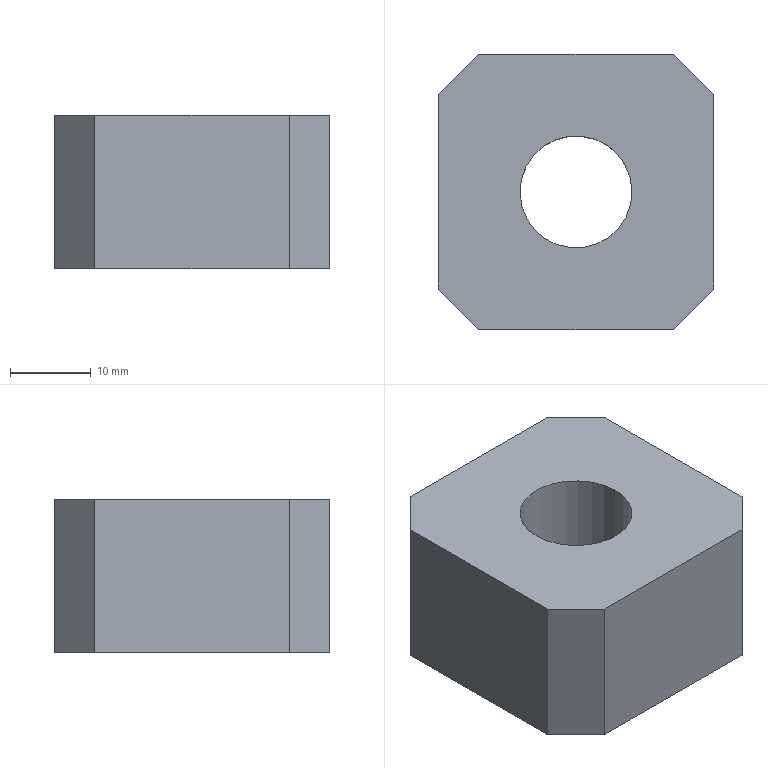Part | STEP file | SN10_002_008-07_PLACA | 1 solid | 11 faces | box 34 x 34 x 19 mm | volume 18158 mm3 | plane 10 | cylinder 1 | commonest cylinder face diameters 13.835 x1
STEP:
#1=CARTESIAN_POINT('',(0.,0.,0.));
#2=DIRECTION('',(0.,0.,1.));
#3=DIRECTION('',(1.,0.,0.));
#4=AXIS2_PLACEMENT_3D('',#1,#2,#3);
#5=CARTESIAN_POINT('',(6.071,3.316,-19.));
#6=VERTEX_POINT('',#5);
#7=CARTESIAN_POINT('',(0.,0.,-19.));
#8=DIRECTION('',(0.,0.,1.));
#9=DIRECTION('',(1.,0.,0.));
#10=AXIS2_PLACEMENT_3D('',#7,#8,#9);
#11=CIRCLE('',#10,6.918);
#12=CARTESIAN_POINT('',(0.,0.,-18.9));
#13=DIRECTION('',(0.,0.,1.));
#14=DIRECTION('',(0.8776,0.4794,0.));
#15=AXIS2_PLACEMENT_3D('',#12,#13,#14);
#16=CYLINDRICAL_SURFACE('',#15,6.918);
#17=CARTESIAN_POINT('',(-0.5,-0.1));
#18=DIRECTION('',(1.,0.));
#19=VECTOR('',#18,1.);
#20=LINE('',#17,#19);
#21=(GEOMETRIC_REPRESENTATION_CONTEXT(2)PARAMETRIC_REPRESENTATION_CONTEXT()REPRESENTATION_CONTEXT('',''));
#22=DEFINITIONAL_REPRESENTATION('',(#20),#21);
#23=PCURVE('',#16,#22);
#24=CARTESIAN_POINT('',(0.,0.,-19.));
#25=DIRECTION('',(0.,0.,1.));
#26=DIRECTION('',(1.,0.,0.));
#27=AXIS2_PLACEMENT_3D('',#24,#25,#26);
#28=PLANE('',#27);
#29=CARTESIAN_POINT('',(0.,0.));
#30=DIRECTION('',(1.,0.));
#31=AXIS2_PLACEMENT_2D('',#29,#30);
#32=CIRCLE('',#31,6.918);
#33=(GEOMETRIC_REPRESENTATION_CONTEXT(2)PARAMETRIC_REPRESENTATION_CONTEXT()REPRESENTATION_CONTEXT('',''));
#34=DEFINITIONAL_REPRESENTATION('',(#32),#33);
#35=PCURVE('',#28,#34);
#36=SURFACE_CURVE('',#11,(#23,#35),.PCURVE_S1.);
#37=EDGE_CURVE('',#6,#6,#36,.T.);
#38=ORIENTED_EDGE('',*,*,#37,.T.);
#39=CARTESIAN_POINT('',(6.071,3.316,0.));
#40=VERTEX_POINT('',#39);
#41=CARTESIAN_POINT('',(6.071,3.316,-19.));
#42=CARTESIAN_POINT('',(6.071,3.316,0.));
#43=B_SPLINE_CURVE_WITH_KNOTS('',1,(#41,#42),.UNSPECIFIED.,.F.,.F.,(2,2),(-0.1,18.9),.PIECEWISE_BEZIER_KNOTS.);
#44=CARTESIAN_POINT('',(6.283,0.));
#45=DIRECTION('',(0.,1.));
#46=VECTOR('',#45,1.);
#47=LINE('',#44,#46);
#48=(GEOMETRIC_REPRESENTATION_CONTEXT(2)PARAMETRIC_REPRESENTATION_CONTEXT()REPRESENTATION_CONTEXT('',''));
#49=DEFINITIONAL_REPRESENTATION('',(#47),#48);
#50=PCURVE('',#16,#49);
#51=CARTESIAN_POINT('',(0.,0.));
#52=DIRECTION('',(0.,1.));
#53=VECTOR('',#52,1.);
#54=LINE('',#51,#53);
#55=(GEOMETRIC_REPRESENTATION_CONTEXT(2)PARAMETRIC_REPRESENTATION_CONTEXT()REPRESENTATION_CONTEXT('',''));
#56=DEFINITIONAL_REPRESENTATION('',(#54),#55);
#57=PCURVE('',#16,#56);
#58=SEAM_CURVE('',#43,(#50,#57),.PCURVE_S1.);
#59=EDGE_CURVE('',#6,#40,#58,.T.);
#60=ORIENTED_EDGE('',*,*,#59,.T.);
#61=CARTESIAN_POINT('',(0.,0.,0.));
#62=DIRECTION('',(0.,0.,1.));
#63=DIRECTION('',(1.,0.,0.));
#64=AXIS2_PLACEMENT_3D('',#61,#62,#63);
#65=CIRCLE('',#64,6.918);
#66=CARTESIAN_POINT('',(-0.5,18.9));
#67=DIRECTION('',(1.,0.));
#68=VECTOR('',#67,1.);
#69=LINE('',#66,#68);
#70=(GEOMETRIC_REPRESENTATION_CONTEXT(2)PARAMETRIC_REPRESENTATION_CONTEXT()REPRESENTATION_CONTEXT('',''));
#71=DEFINITIONAL_REPRESENTATION('',(#69),#70);
#72=PCURVE('',#16,#71);
#73=CARTESIAN_POINT('',(0.,0.,0.));
#74=DIRECTION('',(0.,0.,1.));
#75=DIRECTION('',(1.,0.,0.));
#76=AXIS2_PLACEMENT_3D('',#73,#74,#75);
#77=PLANE('',#76);
#78=CARTESIAN_POINT('',(0.,0.));
#79=DIRECTION('',(1.,0.));
#80=AXIS2_PLACEMENT_2D('',#78,#79);
#81=CIRCLE('',#80,6.918);
#82=(GEOMETRIC_REPRESENTATION_CONTEXT(2)PARAMETRIC_REPRESENTATION_CONTEXT()REPRESENTATION_CONTEXT('',''));
#83=DEFINITIONAL_REPRESENTATION('',(#81),#82);
#84=PCURVE('',#77,#83);
#85=SURFACE_CURVE('',#65,(#72,#84),.PCURVE_S1.);
#86=EDGE_CURVE('',#40,#40,#85,.T.);
#87=ORIENTED_EDGE('',*,*,#86,.F.);
#88=ORIENTED_EDGE('',*,*,#59,.F.);
#89=EDGE_LOOP('',(#38,#60,#87,#88));
#90=FACE_BOUND('',#89,.F.);
#91=ADVANCED_FACE('',(#90),#16,.F.);
#92=CARTESIAN_POINT('',(-17.,-12.,0.));
#93=VERTEX_POINT('',#92);
#94=CARTESIAN_POINT('',(-17.,12.,0.));
#95=VERTEX_POINT('',#94);
#96=CARTESIAN_POINT('',(-17.,-12.,0.));
#97=DIRECTION('',(0.,1.,0.));
#98=VECTOR('',#97,1.);
#99=LINE('',#96,#98);
#100=CARTESIAN_POINT('',(-17.,-12.));
#101=DIRECTION('',(0.,1.));
#102=VECTOR('',#101,1.);
#103=LINE('',#100,#102);
#104=(GEOMETRIC_REPRESENTATION_CONTEXT(2)PARAMETRIC_REPRESENTATION_CONTEXT()REPRESENTATION_CONTEXT('',''));
#105=DEFINITIONAL_REPRESENTATION('',(#103),#104);
#106=PCURVE('',#77,#105);
#107=CARTESIAN_POINT('',(-17.,-17.,0.));
#108=DIRECTION('',(-1.,0.,0.));
#109=DIRECTION('',(0.,0.,1.));
#110=AXIS2_PLACEMENT_3D('',#107,#108,#109);
#111=PLANE('',#110);
#112=CARTESIAN_POINT('',(0.,5.));
#113=DIRECTION('',(0.,1.));
#114=VECTOR('',#113,1.);
#115=LINE('',#112,#114);
#116=(GEOMETRIC_REPRESENTATION_CONTEXT(2)PARAMETRIC_REPRESENTATION_CONTEXT()REPRESENTATION_CONTEXT('',''));
#117=DEFINITIONAL_REPRESENTATION('',(#115),#116);
#118=PCURVE('',#111,#117);
#119=SURFACE_CURVE('',#99,(#106,#118),.PCURVE_S1.);
#120=EDGE_CURVE('',#93,#95,#119,.T.);
#121=ORIENTED_EDGE('',*,*,#120,.F.);
#122=CARTESIAN_POINT('',(-12.,-17.,0.));
#123=VERTEX_POINT('',#122);
#124=CARTESIAN_POINT('',(-17.,-12.,0.));
#125=DIRECTION('',(0.7071,-0.7071,0.));
#126=VECTOR('',#125,1.);
#127=LINE('',#124,#126);
#128=CARTESIAN_POINT('',(-17.,-12.));
#129=DIRECTION('',(0.7071,-0.7071));
#130=VECTOR('',#129,1.);
#131=LINE('',#128,#130);
#132=(GEOMETRIC_REPRESENTATION_CONTEXT(2)PARAMETRIC_REPRESENTATION_CONTEXT()REPRESENTATION_CONTEXT('',''));
#133=DEFINITIONAL_REPRESENTATION('',(#131),#132);
#134=PCURVE('',#77,#133);
#135=CARTESIAN_POINT('',(-17.,-12.,-22.8));
#136=DIRECTION('',(0.7071,0.7071,0.));
#137=DIRECTION('',(0.,0.,-1.));
#138=AXIS2_PLACEMENT_3D('',#135,#136,#137);
#139=PLANE('',#138);
#140=CARTESIAN_POINT('',(-22.8,0.));
#141=DIRECTION('',(0.,-1.));
#142=VECTOR('',#141,1.);
#143=LINE('',#140,#142);
#144=(GEOMETRIC_REPRESENTATION_CONTEXT(2)PARAMETRIC_REPRESENTATION_CONTEXT()REPRESENTATION_CONTEXT('',''));
#145=DEFINITIONAL_REPRESENTATION('',(#143),#144);
#146=PCURVE('',#139,#145);
#147=SURFACE_CURVE('',#127,(#134,#146),.PCURVE_S1.);
#148=EDGE_CURVE('',#93,#123,#147,.T.);
#149=ORIENTED_EDGE('',*,*,#148,.T.);
#150=CARTESIAN_POINT('',(12.,-17.,0.));
#151=VERTEX_POINT('',#150);
#152=CARTESIAN_POINT('',(12.,-17.,0.));
#153=DIRECTION('',(-1.,0.,0.));
#154=VECTOR('',#153,1.);
#155=LINE('',#152,#154);
#156=CARTESIAN_POINT('',(12.,-17.));
#157=DIRECTION('',(-1.,0.));
#158=VECTOR('',#157,1.);
#159=LINE('',#156,#158);
#160=(GEOMETRIC_REPRESENTATION_CONTEXT(2)PARAMETRIC_REPRESENTATION_CONTEXT()REPRESENTATION_CONTEXT('',''));
#161=DEFINITIONAL_REPRESENTATION('',(#159),#160);
#162=PCURVE('',#77,#161);
#163=CARTESIAN_POINT('',(17.,-17.,0.));
#164=DIRECTION('',(0.,-1.,0.));
#165=DIRECTION('',(0.,0.,-1.));
#166=AXIS2_PLACEMENT_3D('',#163,#164,#165);
#167=PLANE('',#166);
#168=CARTESIAN_POINT('',(0.,-5.));
#169=DIRECTION('',(0.,-1.));
#170=VECTOR('',#169,1.);
#171=LINE('',#168,#170);
#172=(GEOMETRIC_REPRESENTATION_CONTEXT(2)PARAMETRIC_REPRESENTATION_CONTEXT()REPRESENTATION_CONTEXT('',''));
#173=DEFINITIONAL_REPRESENTATION('',(#171),#172);
#174=PCURVE('',#167,#173);
#175=SURFACE_CURVE('',#155,(#162,#174),.PCURVE_S1.);
#176=EDGE_CURVE('',#151,#123,#175,.T.);
#177=ORIENTED_EDGE('',*,*,#176,.F.);
#178=CARTESIAN_POINT('',(17.,-12.,0.));
#179=VERTEX_POINT('',#178);
#180=CARTESIAN_POINT('',(17.,-12.,0.));
#181=DIRECTION('',(-0.7071,-0.7071,0.));
#182=VECTOR('',#181,1.);
#183=LINE('',#180,#182);
#184=CARTESIAN_POINT('',(17.,-12.));
#185=DIRECTION('',(-0.7071,-0.7071));
#186=VECTOR('',#185,1.);
#187=LINE('',#184,#186);
#188=(GEOMETRIC_REPRESENTATION_CONTEXT(2)PARAMETRIC_REPRESENTATION_CONTEXT()REPRESENTATION_CONTEXT('',''));
#189=DEFINITIONAL_REPRESENTATION('',(#187),#188);
#190=PCURVE('',#77,#189);
#191=CARTESIAN_POINT('',(17.,-12.,3.8));
#192=DIRECTION('',(-0.7071,0.7071,0.));
#193=DIRECTION('',(0.,0.,1.));
#194=AXIS2_PLACEMENT_3D('',#191,#192,#193);
#195=PLANE('',#194);
#196=CARTESIAN_POINT('',(-3.8,0.));
#197=DIRECTION('',(0.,-1.));
#198=VECTOR('',#197,1.);
#199=LINE('',#196,#198);
#200=(GEOMETRIC_REPRESENTATION_CONTEXT(2)PARAMETRIC_REPRESENTATION_CONTEXT()REPRESENTATION_CONTEXT('',''));
#201=DEFINITIONAL_REPRESENTATION('',(#199),#200);
#202=PCURVE('',#195,#201);
#203=SURFACE_CURVE('',#183,(#190,#202),.PCURVE_S1.);
#204=EDGE_CURVE('',#179,#151,#203,.T.);
#205=ORIENTED_EDGE('',*,*,#204,.F.);
#206=CARTESIAN_POINT('',(17.,12.,0.));
#207=VERTEX_POINT('',#206);
#208=CARTESIAN_POINT('',(17.,12.,0.));
#209=DIRECTION('',(0.,-1.,0.));
#210=VECTOR('',#209,1.);
#211=LINE('',#208,#210);
#212=CARTESIAN_POINT('',(17.,12.));
#213=DIRECTION('',(0.,-1.));
#214=VECTOR('',#213,1.);
#215=LINE('',#212,#214);
#216=(GEOMETRIC_REPRESENTATION_CONTEXT(2)PARAMETRIC_REPRESENTATION_CONTEXT()REPRESENTATION_CONTEXT('',''));
#217=DEFINITIONAL_REPRESENTATION('',(#215),#216);
#218=PCURVE('',#77,#217);
#219=CARTESIAN_POINT('',(17.,17.,0.));
#220=DIRECTION('',(1.,0.,0.));
#221=DIRECTION('',(0.,0.,-1.));
#222=AXIS2_PLACEMENT_3D('',#219,#220,#221);
#223=PLANE('',#222);
#224=CARTESIAN_POINT('',(0.,-5.));
#225=DIRECTION('',(0.,-1.));
#226=VECTOR('',#225,1.);
#227=LINE('',#224,#226);
#228=(GEOMETRIC_REPRESENTATION_CONTEXT(2)PARAMETRIC_REPRESENTATION_CONTEXT()REPRESENTATION_CONTEXT('',''));
#229=DEFINITIONAL_REPRESENTATION('',(#227),#228);
#230=PCURVE('',#223,#229);
#231=SURFACE_CURVE('',#211,(#218,#230),.PCURVE_S1.);
#232=EDGE_CURVE('',#207,#179,#231,.T.);
#233=ORIENTED_EDGE('',*,*,#232,.F.);
#234=CARTESIAN_POINT('',(12.,17.,0.));
#235=VERTEX_POINT('',#234);
#236=CARTESIAN_POINT('',(12.,17.,0.));
#237=DIRECTION('',(0.7071,-0.7071,0.));
#238=VECTOR('',#237,1.);
#239=LINE('',#236,#238);
#240=CARTESIAN_POINT('',(12.,17.));
#241=DIRECTION('',(0.7071,-0.7071));
#242=VECTOR('',#241,1.);
#243=LINE('',#240,#242);
#244=(GEOMETRIC_REPRESENTATION_CONTEXT(2)PARAMETRIC_REPRESENTATION_CONTEXT()REPRESENTATION_CONTEXT('',''));
#245=DEFINITIONAL_REPRESENTATION('',(#243),#244);
#246=PCURVE('',#77,#245);
#247=CARTESIAN_POINT('',(17.,12.,-22.8));
#248=DIRECTION('',(-0.7071,-0.7071,0.));
#249=DIRECTION('',(0.,0.,1.));
#250=AXIS2_PLACEMENT_3D('',#247,#248,#249);
#251=PLANE('',#250);
#252=CARTESIAN_POINT('',(22.8,7.071));
#253=DIRECTION('',(0.,-1.));
#254=VECTOR('',#253,1.);
#255=LINE('',#252,#254);
#256=(GEOMETRIC_REPRESENTATION_CONTEXT(2)PARAMETRIC_REPRESENTATION_CONTEXT()REPRESENTATION_CONTEXT('',''));
#257=DEFINITIONAL_REPRESENTATION('',(#255),#256);
#258=PCURVE('',#251,#257);
#259=SURFACE_CURVE('',#239,(#246,#258),.PCURVE_S1.);
#260=EDGE_CURVE('',#235,#207,#259,.T.);
#261=ORIENTED_EDGE('',*,*,#260,.F.);
#262=CARTESIAN_POINT('',(-12.,17.,0.));
#263=VERTEX_POINT('',#262);
#264=CARTESIAN_POINT('',(-12.,17.,0.));
#265=DIRECTION('',(1.,0.,0.));
#266=VECTOR('',#265,1.);
#267=LINE('',#264,#266);
#268=CARTESIAN_POINT('',(-12.,17.));
#269=DIRECTION('',(1.,0.));
#270=VECTOR('',#269,1.);
#271=LINE('',#268,#270);
#272=(GEOMETRIC_REPRESENTATION_CONTEXT(2)PARAMETRIC_REPRESENTATION_CONTEXT()REPRESENTATION_CONTEXT('',''));
#273=DEFINITIONAL_REPRESENTATION('',(#271),#272);
#274=PCURVE('',#77,#273);
#275=CARTESIAN_POINT('',(-17.,17.,0.));
#276=DIRECTION('',(0.,1.,0.));
#277=DIRECTION('',(0.,0.,1.));
#278=AXIS2_PLACEMENT_3D('',#275,#276,#277);
#279=PLANE('',#278);
#280=CARTESIAN_POINT('',(0.,5.));
#281=DIRECTION('',(0.,1.));
#282=VECTOR('',#281,1.);
#283=LINE('',#280,#282);
#284=(GEOMETRIC_REPRESENTATION_CONTEXT(2)PARAMETRIC_REPRESENTATION_CONTEXT()REPRESENTATION_CONTEXT('',''));
#285=DEFINITIONAL_REPRESENTATION('',(#283),#284);
#286=PCURVE('',#279,#285);
#287=SURFACE_CURVE('',#267,(#274,#286),.PCURVE_S1.);
#288=EDGE_CURVE('',#263,#235,#287,.T.);
#289=ORIENTED_EDGE('',*,*,#288,.F.);
#290=CARTESIAN_POINT('',(-17.,12.,0.));
#291=DIRECTION('',(0.7071,0.7071,0.));
#292=VECTOR('',#291,1.);
#293=LINE('',#290,#292);
#294=CARTESIAN_POINT('',(-17.,12.));
#295=DIRECTION('',(0.7071,0.7071));
#296=VECTOR('',#295,1.);
#297=LINE('',#294,#296);
#298=(GEOMETRIC_REPRESENTATION_CONTEXT(2)PARAMETRIC_REPRESENTATION_CONTEXT()REPRESENTATION_CONTEXT('',''));
#299=DEFINITIONAL_REPRESENTATION('',(#297),#298);
#300=PCURVE('',#77,#299);
#301=CARTESIAN_POINT('',(-17.,12.,3.8));
#302=DIRECTION('',(0.7071,-0.7071,0.));
#303=DIRECTION('',(0.,0.,-1.));
#304=AXIS2_PLACEMENT_3D('',#301,#302,#303);
#305=PLANE('',#304);
#306=CARTESIAN_POINT('',(3.8,0.));
#307=DIRECTION('',(0.,1.));
#308=VECTOR('',#307,1.);
#309=LINE('',#306,#308);
#310=(GEOMETRIC_REPRESENTATION_CONTEXT(2)PARAMETRIC_REPRESENTATION_CONTEXT()REPRESENTATION_CONTEXT('',''));
#311=DEFINITIONAL_REPRESENTATION('',(#309),#310);
#312=PCURVE('',#305,#311);
#313=SURFACE_CURVE('',#293,(#300,#312),.PCURVE_S1.);
#314=EDGE_CURVE('',#95,#263,#313,.T.);
#315=ORIENTED_EDGE('',*,*,#314,.F.);
#316=EDGE_LOOP('',(#121,#149,#177,#205,#233,#261,#289,#315));
#317=FACE_BOUND('',#316,.T.);
#318=ORIENTED_EDGE('',*,*,#86,.F.);
#319=EDGE_LOOP('',(#318));
#320=FACE_BOUND('',#319,.T.);
#321=ADVANCED_FACE('',(#317,#320),#77,.T.);
#322=CARTESIAN_POINT('',(-17.,-12.,-19.));
#323=VERTEX_POINT('',#322);
#324=CARTESIAN_POINT('',(-17.,12.,-19.));
#325=VERTEX_POINT('',#324);
#326=CARTESIAN_POINT('',(-17.,-12.,-19.));
#327=DIRECTION('',(0.,1.,0.));
#328=VECTOR('',#327,1.);
#329=LINE('',#326,#328);
#330=CARTESIAN_POINT('',(-19.,5.));
#331=DIRECTION('',(0.,1.));
#332=VECTOR('',#331,1.);
#333=LINE('',#330,#332);
#334=(GEOMETRIC_REPRESENTATION_CONTEXT(2)PARAMETRIC_REPRESENTATION_CONTEXT()REPRESENTATION_CONTEXT('',''));
#335=DEFINITIONAL_REPRESENTATION('',(#333),#334);
#336=PCURVE('',#111,#335);
#337=CARTESIAN_POINT('',(-17.,-12.));
#338=DIRECTION('',(0.,1.));
#339=VECTOR('',#338,1.);
#340=LINE('',#337,#339);
#341=(GEOMETRIC_REPRESENTATION_CONTEXT(2)PARAMETRIC_REPRESENTATION_CONTEXT()REPRESENTATION_CONTEXT('',''));
#342=DEFINITIONAL_REPRESENTATION('',(#340),#341);
#343=PCURVE('',#28,#342);
#344=SURFACE_CURVE('',#329,(#336,#343),.PCURVE_S1.);
#345=EDGE_CURVE('',#323,#325,#344,.T.);
#346=ORIENTED_EDGE('',*,*,#345,.F.);
#347=CARTESIAN_POINT('',(-17.,-12.,-19.));
#348=DIRECTION('',(0.,0.,1.));
#349=VECTOR('',#348,1.);
#350=LINE('',#347,#349);
#351=CARTESIAN_POINT('',(-19.,5.));
#352=DIRECTION('',(1.,0.));
#353=VECTOR('',#352,1.);
#354=LINE('',#351,#353);
#355=(GEOMETRIC_REPRESENTATION_CONTEXT(2)PARAMETRIC_REPRESENTATION_CONTEXT()REPRESENTATION_CONTEXT('',''));
#356=DEFINITIONAL_REPRESENTATION('',(#354),#355);
#357=PCURVE('',#111,#356);
#358=CARTESIAN_POINT('',(-3.8,0.));
#359=DIRECTION('',(-1.,0.));
#360=VECTOR('',#359,1.);
#361=LINE('',#358,#360);
#362=(GEOMETRIC_REPRESENTATION_CONTEXT(2)PARAMETRIC_REPRESENTATION_CONTEXT()REPRESENTATION_CONTEXT('',''));
#363=DEFINITIONAL_REPRESENTATION('',(#361),#362);
#364=PCURVE('',#139,#363);
#365=SURFACE_CURVE('',#350,(#357,#364),.PCURVE_S1.);
#366=EDGE_CURVE('',#323,#93,#365,.T.);
#367=ORIENTED_EDGE('',*,*,#366,.T.);
#368=ORIENTED_EDGE('',*,*,#120,.T.);
#369=CARTESIAN_POINT('',(-17.,12.,0.));
#370=DIRECTION('',(0.,0.,-1.));
#371=VECTOR('',#370,1.);
#372=LINE('',#369,#371);
#373=CARTESIAN_POINT('',(0.,29.));
#374=DIRECTION('',(-1.,0.));
#375=VECTOR('',#374,1.);
#376=LINE('',#373,#375);
#377=(GEOMETRIC_REPRESENTATION_CONTEXT(2)PARAMETRIC_REPRESENTATION_CONTEXT()REPRESENTATION_CONTEXT('',''));
#378=DEFINITIONAL_REPRESENTATION('',(#376),#377);
#379=PCURVE('',#111,#378);
#380=CARTESIAN_POINT('',(3.8,0.));
#381=DIRECTION('',(1.,0.));
#382=VECTOR('',#381,1.);
#383=LINE('',#380,#382);
#384=(GEOMETRIC_REPRESENTATION_CONTEXT(2)PARAMETRIC_REPRESENTATION_CONTEXT()REPRESENTATION_CONTEXT('',''));
#385=DEFINITIONAL_REPRESENTATION('',(#383),#384);
#386=PCURVE('',#305,#385);
#387=SURFACE_CURVE('',#372,(#379,#386),.PCURVE_S1.);
#388=EDGE_CURVE('',#95,#325,#387,.T.);
#389=ORIENTED_EDGE('',*,*,#388,.T.);
#390=EDGE_LOOP('',(#346,#367,#368,#389));
#391=FACE_BOUND('',#390,.T.);
#392=ADVANCED_FACE('',(#391),#111,.T.);
#393=CARTESIAN_POINT('',(12.,-17.,-19.));
#394=VERTEX_POINT('',#393);
#395=CARTESIAN_POINT('',(-12.,-17.,-19.));
#396=VERTEX_POINT('',#395);
#397=CARTESIAN_POINT('',(12.,-17.,-19.));
#398=DIRECTION('',(-1.,0.,0.));
#399=VECTOR('',#398,1.);
#400=LINE('',#397,#399);
#401=CARTESIAN_POINT('',(19.,-5.));
#402=DIRECTION('',(0.,-1.));
#403=VECTOR('',#402,1.);
#404=LINE('',#401,#403);
#405=(GEOMETRIC_REPRESENTATION_CONTEXT(2)PARAMETRIC_REPRESENTATION_CONTEXT()REPRESENTATION_CONTEXT('',''));
#406=DEFINITIONAL_REPRESENTATION('',(#404),#405);
#407=PCURVE('',#167,#406);
#408=CARTESIAN_POINT('',(12.,-17.));
#409=DIRECTION('',(-1.,0.));
#410=VECTOR('',#409,1.);
#411=LINE('',#408,#410);
#412=(GEOMETRIC_REPRESENTATION_CONTEXT(2)PARAMETRIC_REPRESENTATION_CONTEXT()REPRESENTATION_CONTEXT('',''));
#413=DEFINITIONAL_REPRESENTATION('',(#411),#412);
#414=PCURVE('',#28,#413);
#415=SURFACE_CURVE('',#400,(#407,#414),.PCURVE_S1.);
#416=EDGE_CURVE('',#394,#396,#415,.T.);
#417=ORIENTED_EDGE('',*,*,#416,.F.);
#418=CARTESIAN_POINT('',(12.,-17.,0.));
#419=DIRECTION('',(0.,0.,-1.));
#420=VECTOR('',#419,1.);
#421=LINE('',#418,#420);
#422=CARTESIAN_POINT('',(0.,-5.));
#423=DIRECTION('',(1.,0.));
#424=VECTOR('',#423,1.);
#425=LINE('',#422,#424);
#426=(GEOMETRIC_REPRESENTATION_CONTEXT(2)PARAMETRIC_REPRESENTATION_CONTEXT()REPRESENTATION_CONTEXT('',''));
#427=DEFINITIONAL_REPRESENTATION('',(#425),#426);
#428=PCURVE('',#167,#427);
#429=CARTESIAN_POINT('',(-3.8,-7.071));
#430=DIRECTION('',(-1.,0.));
#431=VECTOR('',#430,1.);
#432=LINE('',#429,#431);
#433=(GEOMETRIC_REPRESENTATION_CONTEXT(2)PARAMETRIC_REPRESENTATION_CONTEXT()REPRESENTATION_CONTEXT('',''));
#434=DEFINITIONAL_REPRESENTATION('',(#432),#433);
#435=PCURVE('',#195,#434);
#436=SURFACE_CURVE('',#421,(#428,#435),.PCURVE_S1.);
#437=EDGE_CURVE('',#151,#394,#436,.T.);
#438=ORIENTED_EDGE('',*,*,#437,.F.);
#439=ORIENTED_EDGE('',*,*,#176,.T.);
#440=CARTESIAN_POINT('',(-12.,-17.,-19.));
#441=DIRECTION('',(0.,0.,1.));
#442=VECTOR('',#441,1.);
#443=LINE('',#440,#442);
#444=CARTESIAN_POINT('',(19.,-29.));
#445=DIRECTION('',(-1.,0.));
#446=VECTOR('',#445,1.);
#447=LINE('',#444,#446);
#448=(GEOMETRIC_REPRESENTATION_CONTEXT(2)PARAMETRIC_REPRESENTATION_CONTEXT()REPRESENTATION_CONTEXT('',''));
#449=DEFINITIONAL_REPRESENTATION('',(#447),#448);
#450=PCURVE('',#167,#449);
#451=CARTESIAN_POINT('',(-3.8,-7.071));
#452=DIRECTION('',(-1.,0.));
#453=VECTOR('',#452,1.);
#454=LINE('',#451,#453);
#455=(GEOMETRIC_REPRESENTATION_CONTEXT(2)PARAMETRIC_REPRESENTATION_CONTEXT()REPRESENTATION_CONTEXT('',''));
#456=DEFINITIONAL_REPRESENTATION('',(#454),#455);
#457=PCURVE('',#139,#456);
#458=SURFACE_CURVE('',#443,(#450,#457),.PCURVE_S1.);
#459=EDGE_CURVE('',#396,#123,#458,.T.);
#460=ORIENTED_EDGE('',*,*,#459,.F.);
#461=EDGE_LOOP('',(#417,#438,#439,#460));
#462=FACE_BOUND('',#461,.T.);
#463=ADVANCED_FACE('',(#462),#167,.T.);
#464=CARTESIAN_POINT('',(17.,12.,-19.));
#465=VERTEX_POINT('',#464);
#466=CARTESIAN_POINT('',(17.,-12.,-19.));
#467=VERTEX_POINT('',#466);
#468=CARTESIAN_POINT('',(17.,12.,-19.));
#469=DIRECTION('',(0.,-1.,0.));
#470=VECTOR('',#469,1.);
#471=LINE('',#468,#470);
#472=CARTESIAN_POINT('',(19.,-5.));
#473=DIRECTION('',(0.,-1.));
#474=VECTOR('',#473,1.);
#475=LINE('',#472,#474);
#476=(GEOMETRIC_REPRESENTATION_CONTEXT(2)PARAMETRIC_REPRESENTATION_CONTEXT()REPRESENTATION_CONTEXT('',''));
#477=DEFINITIONAL_REPRESENTATION('',(#475),#476);
#478=PCURVE('',#223,#477);
#479=CARTESIAN_POINT('',(17.,12.));
#480=DIRECTION('',(0.,-1.));
#481=VECTOR('',#480,1.);
#482=LINE('',#479,#481);
#483=(GEOMETRIC_REPRESENTATION_CONTEXT(2)PARAMETRIC_REPRESENTATION_CONTEXT()REPRESENTATION_CONTEXT('',''));
#484=DEFINITIONAL_REPRESENTATION('',(#482),#483);
#485=PCURVE('',#28,#484);
#486=SURFACE_CURVE('',#471,(#478,#485),.PCURVE_S1.);
#487=EDGE_CURVE('',#465,#467,#486,.T.);
#488=ORIENTED_EDGE('',*,*,#487,.F.);
#489=CARTESIAN_POINT('',(17.,12.,-19.));
#490=DIRECTION('',(0.,0.,1.));
#491=VECTOR('',#490,1.);
#492=LINE('',#489,#491);
#493=CARTESIAN_POINT('',(19.,-5.));
#494=DIRECTION('',(-1.,0.));
#495=VECTOR('',#494,1.);
#496=LINE('',#493,#495);
#497=(GEOMETRIC_REPRESENTATION_CONTEXT(2)PARAMETRIC_REPRESENTATION_CONTEXT()REPRESENTATION_CONTEXT('',''));
#498=DEFINITIONAL_REPRESENTATION('',(#496),#497);
#499=PCURVE('',#223,#498);
#500=CARTESIAN_POINT('',(3.8,0.));
#501=DIRECTION('',(1.,0.));
#502=VECTOR('',#501,1.);
#503=LINE('',#500,#502);
#504=(GEOMETRIC_REPRESENTATION_CONTEXT(2)PARAMETRIC_REPRESENTATION_CONTEXT()REPRESENTATION_CONTEXT('',''));
#505=DEFINITIONAL_REPRESENTATION('',(#503),#504);
#506=PCURVE('',#251,#505);
#507=SURFACE_CURVE('',#492,(#499,#506),.PCURVE_S1.);
#508=EDGE_CURVE('',#465,#207,#507,.T.);
#509=ORIENTED_EDGE('',*,*,#508,.T.);
#510=ORIENTED_EDGE('',*,*,#232,.T.);
#511=CARTESIAN_POINT('',(17.,-12.,0.));
#512=DIRECTION('',(0.,0.,-1.));
#513=VECTOR('',#512,1.);
#514=LINE('',#511,#513);
#515=CARTESIAN_POINT('',(0.,-29.));
#516=DIRECTION('',(1.,0.));
#517=VECTOR('',#516,1.);
#518=LINE('',#515,#517);
#519=(GEOMETRIC_REPRESENTATION_CONTEXT(2)PARAMETRIC_REPRESENTATION_CONTEXT()REPRESENTATION_CONTEXT('',''));
#520=DEFINITIONAL_REPRESENTATION('',(#518),#519);
#521=PCURVE('',#223,#520);
#522=CARTESIAN_POINT('',(-3.8,0.));
#523=DIRECTION('',(-1.,0.));
#524=VECTOR('',#523,1.);
#525=LINE('',#522,#524);
#526=(GEOMETRIC_REPRESENTATION_CONTEXT(2)PARAMETRIC_REPRESENTATION_CONTEXT()REPRESENTATION_CONTEXT('',''));
#527=DEFINITIONAL_REPRESENTATION('',(#525),#526);
#528=PCURVE('',#195,#527);
#529=SURFACE_CURVE('',#514,(#521,#528),.PCURVE_S1.);
#530=EDGE_CURVE('',#179,#467,#529,.T.);
#531=ORIENTED_EDGE('',*,*,#530,.T.);
#532=EDGE_LOOP('',(#488,#509,#510,#531));
#533=FACE_BOUND('',#532,.T.);
#534=ADVANCED_FACE('',(#533),#223,.T.);
#535=ORIENTED_EDGE('',*,*,#288,.T.);
#536=CARTESIAN_POINT('',(12.,17.,-19.));
#537=VERTEX_POINT('',#536);
#538=CARTESIAN_POINT('',(12.,17.,-19.));
#539=DIRECTION('',(0.,0.,1.));
#540=VECTOR('',#539,1.);
#541=LINE('',#538,#540);
#542=CARTESIAN_POINT('',(-19.,29.));
#543=DIRECTION('',(1.,0.));
#544=VECTOR('',#543,1.);
#545=LINE('',#542,#544);
#546=(GEOMETRIC_REPRESENTATION_CONTEXT(2)PARAMETRIC_REPRESENTATION_CONTEXT()REPRESENTATION_CONTEXT('',''));
#547=DEFINITIONAL_REPRESENTATION('',(#545),#546);
#548=PCURVE('',#279,#547);
#549=CARTESIAN_POINT('',(3.8,7.071));
#550=DIRECTION('',(1.,0.));
#551=VECTOR('',#550,1.);
#552=LINE('',#549,#551);
#553=(GEOMETRIC_REPRESENTATION_CONTEXT(2)PARAMETRIC_REPRESENTATION_CONTEXT()REPRESENTATION_CONTEXT('',''));
#554=DEFINITIONAL_REPRESENTATION('',(#552),#553);
#555=PCURVE('',#251,#554);
#556=SURFACE_CURVE('',#541,(#548,#555),.PCURVE_S1.);
#557=EDGE_CURVE('',#537,#235,#556,.T.);
#558=ORIENTED_EDGE('',*,*,#557,.F.);
#559=CARTESIAN_POINT('',(-12.,17.,-19.));
#560=VERTEX_POINT('',#559);
#561=CARTESIAN_POINT('',(-12.,17.,-19.));
#562=DIRECTION('',(1.,0.,0.));
#563=VECTOR('',#562,1.);
#564=LINE('',#561,#563);
#565=CARTESIAN_POINT('',(-19.,5.));
#566=DIRECTION('',(0.,1.));
#567=VECTOR('',#566,1.);
#568=LINE('',#565,#567);
#569=(GEOMETRIC_REPRESENTATION_CONTEXT(2)PARAMETRIC_REPRESENTATION_CONTEXT()REPRESENTATION_CONTEXT('',''));
#570=DEFINITIONAL_REPRESENTATION('',(#568),#569);
#571=PCURVE('',#279,#570);
#572=CARTESIAN_POINT('',(-12.,17.));
#573=DIRECTION('',(1.,0.));
#574=VECTOR('',#573,1.);
#575=LINE('',#572,#574);
#576=(GEOMETRIC_REPRESENTATION_CONTEXT(2)PARAMETRIC_REPRESENTATION_CONTEXT()REPRESENTATION_CONTEXT('',''));
#577=DEFINITIONAL_REPRESENTATION('',(#575),#576);
#578=PCURVE('',#28,#577);
#579=SURFACE_CURVE('',#564,(#571,#578),.PCURVE_S1.);
#580=EDGE_CURVE('',#560,#537,#579,.T.);
#581=ORIENTED_EDGE('',*,*,#580,.F.);
#582=CARTESIAN_POINT('',(-12.,17.,0.));
#583=DIRECTION('',(0.,0.,-1.));
#584=VECTOR('',#583,1.);
#585=LINE('',#582,#584);
#586=CARTESIAN_POINT('',(0.,5.));
#587=DIRECTION('',(-1.,0.));
#588=VECTOR('',#587,1.);
#589=LINE('',#586,#588);
#590=(GEOMETRIC_REPRESENTATION_CONTEXT(2)PARAMETRIC_REPRESENTATION_CONTEXT()REPRESENTATION_CONTEXT('',''));
#591=DEFINITIONAL_REPRESENTATION('',(#589),#590);
#592=PCURVE('',#279,#591);
#593=CARTESIAN_POINT('',(3.8,7.071));
#594=DIRECTION('',(1.,0.));
#595=VECTOR('',#594,1.);
#596=LINE('',#593,#595);
#597=(GEOMETRIC_REPRESENTATION_CONTEXT(2)PARAMETRIC_REPRESENTATION_CONTEXT()REPRESENTATION_CONTEXT('',''));
#598=DEFINITIONAL_REPRESENTATION('',(#596),#597);
#599=PCURVE('',#305,#598);
#600=SURFACE_CURVE('',#585,(#592,#599),.PCURVE_S1.);
#601=EDGE_CURVE('',#263,#560,#600,.T.);
#602=ORIENTED_EDGE('',*,*,#601,.F.);
#603=EDGE_LOOP('',(#535,#558,#581,#602));
#604=FACE_BOUND('',#603,.T.);
#605=ADVANCED_FACE('',(#604),#279,.T.);
#606=ORIENTED_EDGE('',*,*,#388,.F.);
#607=ORIENTED_EDGE('',*,*,#314,.T.);
#608=ORIENTED_EDGE('',*,*,#601,.T.);
#609=CARTESIAN_POINT('',(-17.,12.,-19.));
#610=DIRECTION('',(0.7071,0.7071,0.));
#611=VECTOR('',#610,1.);
#612=LINE('',#609,#611);
#613=CARTESIAN_POINT('',(22.8,0.));
#614=DIRECTION('',(0.,1.));
#615=VECTOR('',#614,1.);
#616=LINE('',#613,#615);
#617=(GEOMETRIC_REPRESENTATION_CONTEXT(2)PARAMETRIC_REPRESENTATION_CONTEXT()REPRESENTATION_CONTEXT('',''));
#618=DEFINITIONAL_REPRESENTATION('',(#616),#617);
#619=PCURVE('',#305,#618);
#620=CARTESIAN_POINT('',(-17.,12.));
#621=DIRECTION('',(0.7071,0.7071));
#622=VECTOR('',#621,1.);
#623=LINE('',#620,#622);
#624=(GEOMETRIC_REPRESENTATION_CONTEXT(2)PARAMETRIC_REPRESENTATION_CONTEXT()REPRESENTATION_CONTEXT('',''));
#625=DEFINITIONAL_REPRESENTATION('',(#623),#624);
#626=PCURVE('',#28,#625);
#627=SURFACE_CURVE('',#612,(#619,#626),.PCURVE_S1.);
#628=EDGE_CURVE('',#325,#560,#627,.T.);
#629=ORIENTED_EDGE('',*,*,#628,.F.);
#630=EDGE_LOOP('',(#606,#607,#608,#629));
#631=FACE_BOUND('',#630,.T.);
#632=ADVANCED_FACE('',(#631),#305,.F.);
#633=ORIENTED_EDGE('',*,*,#557,.T.);
#634=ORIENTED_EDGE('',*,*,#260,.T.);
#635=ORIENTED_EDGE('',*,*,#508,.F.);
#636=CARTESIAN_POINT('',(17.,12.,-19.));
#637=DIRECTION('',(-0.7071,0.7071,0.));
#638=VECTOR('',#637,1.);
#639=LINE('',#636,#638);
#640=CARTESIAN_POINT('',(3.8,0.));
#641=DIRECTION('',(0.,1.));
#642=VECTOR('',#641,1.);
#643=LINE('',#640,#642);
#644=(GEOMETRIC_REPRESENTATION_CONTEXT(2)PARAMETRIC_REPRESENTATION_CONTEXT()REPRESENTATION_CONTEXT('',''));
#645=DEFINITIONAL_REPRESENTATION('',(#643),#644);
#646=PCURVE('',#251,#645);
#647=CARTESIAN_POINT('',(17.,12.));
#648=DIRECTION('',(-0.7071,0.7071));
#649=VECTOR('',#648,1.);
#650=LINE('',#647,#649);
#651=(GEOMETRIC_REPRESENTATION_CONTEXT(2)PARAMETRIC_REPRESENTATION_CONTEXT()REPRESENTATION_CONTEXT('',''));
#652=DEFINITIONAL_REPRESENTATION('',(#650),#651);
#653=PCURVE('',#28,#652);
#654=SURFACE_CURVE('',#639,(#646,#653),.PCURVE_S1.);
#655=EDGE_CURVE('',#465,#537,#654,.T.);
#656=ORIENTED_EDGE('',*,*,#655,.T.);
#657=EDGE_LOOP('',(#633,#634,#635,#656));
#658=FACE_BOUND('',#657,.T.);
#659=ADVANCED_FACE('',(#658),#251,.F.);
#660=ORIENTED_EDGE('',*,*,#530,.F.);
#661=ORIENTED_EDGE('',*,*,#204,.T.);
#662=ORIENTED_EDGE('',*,*,#437,.T.);
#663=CARTESIAN_POINT('',(17.,-12.,-19.));
#664=DIRECTION('',(-0.7071,-0.7071,0.));
#665=VECTOR('',#664,1.);
#666=LINE('',#663,#665);
#667=CARTESIAN_POINT('',(-22.8,0.));
#668=DIRECTION('',(0.,-1.));
#669=VECTOR('',#668,1.);
#670=LINE('',#667,#669);
#671=(GEOMETRIC_REPRESENTATION_CONTEXT(2)PARAMETRIC_REPRESENTATION_CONTEXT()REPRESENTATION_CONTEXT('',''));
#672=DEFINITIONAL_REPRESENTATION('',(#670),#671);
#673=PCURVE('',#195,#672);
#674=CARTESIAN_POINT('',(17.,-12.));
#675=DIRECTION('',(-0.7071,-0.7071));
#676=VECTOR('',#675,1.);
#677=LINE('',#674,#676);
#678=(GEOMETRIC_REPRESENTATION_CONTEXT(2)PARAMETRIC_REPRESENTATION_CONTEXT()REPRESENTATION_CONTEXT('',''));
#679=DEFINITIONAL_REPRESENTATION('',(#677),#678);
#680=PCURVE('',#28,#679);
#681=SURFACE_CURVE('',#666,(#673,#680),.PCURVE_S1.);
#682=EDGE_CURVE('',#467,#394,#681,.T.);
#683=ORIENTED_EDGE('',*,*,#682,.F.);
#684=EDGE_LOOP('',(#660,#661,#662,#683));
#685=FACE_BOUND('',#684,.T.);
#686=ADVANCED_FACE('',(#685),#195,.F.);
#687=ORIENTED_EDGE('',*,*,#459,.T.);
#688=ORIENTED_EDGE('',*,*,#148,.F.);
#689=ORIENTED_EDGE('',*,*,#366,.F.);
#690=CARTESIAN_POINT('',(-17.,-12.,-19.));
#691=DIRECTION('',(0.7071,-0.7071,0.));
#692=VECTOR('',#691,1.);
#693=LINE('',#690,#692);
#694=CARTESIAN_POINT('',(-3.8,0.));
#695=DIRECTION('',(0.,-1.));
#696=VECTOR('',#695,1.);
#697=LINE('',#694,#696);
#698=(GEOMETRIC_REPRESENTATION_CONTEXT(2)PARAMETRIC_REPRESENTATION_CONTEXT()REPRESENTATION_CONTEXT('',''));
#699=DEFINITIONAL_REPRESENTATION('',(#697),#698);
#700=PCURVE('',#139,#699);
#701=CARTESIAN_POINT('',(-17.,-12.));
#702=DIRECTION('',(0.7071,-0.7071));
#703=VECTOR('',#702,1.);
#704=LINE('',#701,#703);
#705=(GEOMETRIC_REPRESENTATION_CONTEXT(2)PARAMETRIC_REPRESENTATION_CONTEXT()REPRESENTATION_CONTEXT('',''));
#706=DEFINITIONAL_REPRESENTATION('',(#704),#705);
#707=PCURVE('',#28,#706);
#708=SURFACE_CURVE('',#693,(#700,#707),.PCURVE_S1.);
#709=EDGE_CURVE('',#323,#396,#708,.T.);
#710=ORIENTED_EDGE('',*,*,#709,.T.);
#711=EDGE_LOOP('',(#687,#688,#689,#710));
#712=FACE_BOUND('',#711,.T.);
#713=ADVANCED_FACE('',(#712),#139,.F.);
#714=ORIENTED_EDGE('',*,*,#628,.T.);
#715=ORIENTED_EDGE('',*,*,#580,.T.);
#716=ORIENTED_EDGE('',*,*,#655,.F.);
#717=ORIENTED_EDGE('',*,*,#487,.T.);
#718=ORIENTED_EDGE('',*,*,#682,.T.);
#719=ORIENTED_EDGE('',*,*,#416,.T.);
#720=ORIENTED_EDGE('',*,*,#709,.F.);
#721=ORIENTED_EDGE('',*,*,#345,.T.);
#722=EDGE_LOOP('',(#714,#715,#716,#717,#718,#719,#720,#721));
#723=FACE_BOUND('',#722,.T.);
#724=ORIENTED_EDGE('',*,*,#37,.T.);
#725=EDGE_LOOP('',(#724));
#726=FACE_BOUND('',#725,.T.);
#727=ADVANCED_FACE('',(#723,#726),#28,.F.);
#728=CLOSED_SHELL('',(#91,#321,#392,#463,#534,#605,#632,#659,#686,#713,#727));
#729=MANIFOLD_SOLID_BREP('',#728);
#730=(LENGTH_UNIT()NAMED_UNIT(*)SI_UNIT(.MILLI.,.METRE.));
#731=UNCERTAINTY_MEASURE_WITH_UNIT(LENGTH_MEASURE(0.000001),#730,'','');
#732=(NAMED_UNIT(*)PLANE_ANGLE_UNIT()SI_UNIT($,.RADIAN.));
#733=(NAMED_UNIT(*)SI_UNIT($,.STERADIAN.)SOLID_ANGLE_UNIT());
#734=(GEOMETRIC_REPRESENTATION_CONTEXT(3)GLOBAL_UNCERTAINTY_ASSIGNED_CONTEXT((#731))GLOBAL_UNIT_ASSIGNED_CONTEXT((#730,#732,#733))REPRESENTATION_CONTEXT('',''));
#735=ADVANCED_BREP_SHAPE_REPRESENTATION('',(#4,#729),#734);